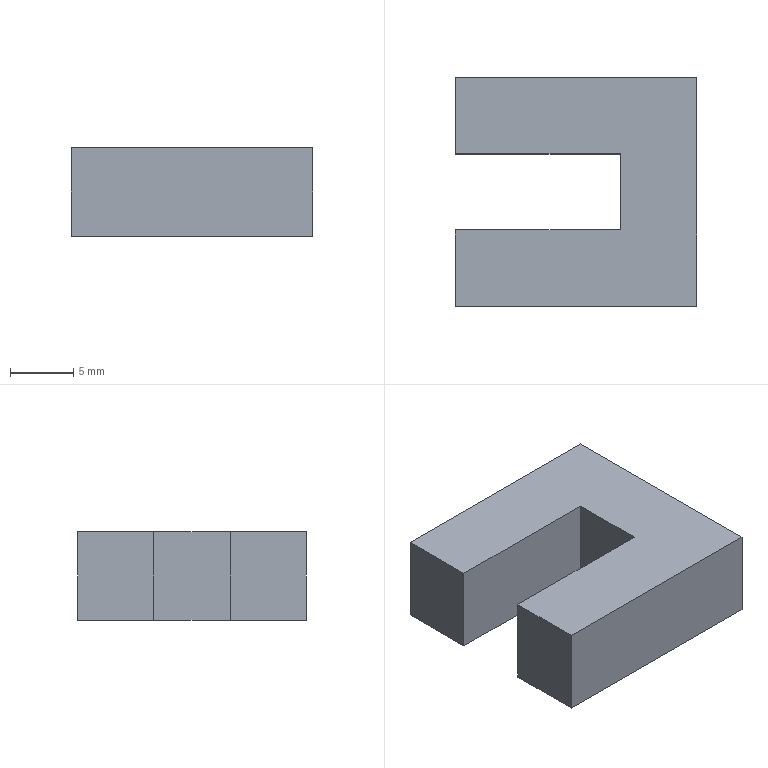Part | SolidWorks | features Extrusion 1 | 1 solid | 10 faces | box 19 x 18 x 7 mm | volume 1848 mm3 | plane 10
STEP:
#1=CARTESIAN_POINT('',(0.,-9.,-3.5));
#2=VERTEX_POINT('',#1);
#3=CARTESIAN_POINT('',(0.,9.,-3.5));
#4=VERTEX_POINT('',#3);
#5=CARTESIAN_POINT('',(0.,0.,-3.5));
#6=DIRECTION('',(0.,1.,0.));
#7=VECTOR('',#6,1000.);
#8=LINE('',#5,#7);
#9=EDGE_CURVE('',#2,#4,#8,.T.);
#10=ORIENTED_EDGE('',*,*,#9,.T.);
#11=CARTESIAN_POINT('',(0.,9.,3.5));
#12=VERTEX_POINT('',#11);
#13=CARTESIAN_POINT('',(0.,9.,3.5));
#14=DIRECTION('',(0.,0.,-1.));
#15=VECTOR('',#14,1000.);
#16=LINE('',#13,#15);
#17=EDGE_CURVE('',#12,#4,#16,.T.);
#18=ORIENTED_EDGE('',*,*,#17,.F.);
#19=CARTESIAN_POINT('',(0.,-9.,3.5));
#20=VERTEX_POINT('',#19);
#21=CARTESIAN_POINT('',(0.,-9.,3.5));
#22=DIRECTION('',(0.,1.,0.));
#23=VECTOR('',#22,1000.);
#24=LINE('',#21,#23);
#25=EDGE_CURVE('',#20,#12,#24,.T.);
#26=ORIENTED_EDGE('',*,*,#25,.F.);
#27=CARTESIAN_POINT('',(0.,-9.,3.5));
#28=DIRECTION('',(0.,0.,-1.));
#29=VECTOR('',#28,1000.);
#30=LINE('',#27,#29);
#31=EDGE_CURVE('',#20,#2,#30,.T.);
#32=ORIENTED_EDGE('',*,*,#31,.T.);
#33=EDGE_LOOP('',(#10,#18,#26,#32));
#34=FACE_OUTER_BOUND('',#33,.T.);
#35=CARTESIAN_POINT('',(0.,0.,3.5));
#36=DIRECTION('',(-1.,0.,0.));
#37=DIRECTION('',(0.,0.,1.));
#38=AXIS2_PLACEMENT_3D('',#35,#36,#37);
#39=PLANE('',#38);
#40=ADVANCED_FACE('',(#34),#39,.F.);
#41=CARTESIAN_POINT('',(-19.,9.,-3.5));
#42=VERTEX_POINT('',#41);
#43=CARTESIAN_POINT('',(0.,9.,-3.5));
#44=DIRECTION('',(-1.,0.,0.));
#45=VECTOR('',#44,1000.);
#46=LINE('',#43,#45);
#47=EDGE_CURVE('',#4,#42,#46,.T.);
#48=ORIENTED_EDGE('',*,*,#47,.T.);
#49=CARTESIAN_POINT('',(-19.,9.,3.5));
#50=VERTEX_POINT('',#49);
#51=CARTESIAN_POINT('',(-19.,9.,3.5));
#52=DIRECTION('',(0.,0.,-1.));
#53=VECTOR('',#52,1000.);
#54=LINE('',#51,#53);
#55=EDGE_CURVE('',#50,#42,#54,.T.);
#56=ORIENTED_EDGE('',*,*,#55,.F.);
#57=CARTESIAN_POINT('',(0.,9.,3.5));
#58=DIRECTION('',(-1.,0.,0.));
#59=VECTOR('',#58,1000.);
#60=LINE('',#57,#59);
#61=EDGE_CURVE('',#12,#50,#60,.T.);
#62=ORIENTED_EDGE('',*,*,#61,.F.);
#63=ORIENTED_EDGE('',*,*,#17,.T.);
#64=EDGE_LOOP('',(#48,#56,#62,#63));
#65=FACE_OUTER_BOUND('',#64,.T.);
#66=CARTESIAN_POINT('',(0.,9.,3.5));
#67=DIRECTION('',(0.,-1.,0.));
#68=DIRECTION('',(1.,0.,0.));
#69=AXIS2_PLACEMENT_3D('',#66,#67,#68);
#70=PLANE('',#69);
#71=ADVANCED_FACE('',(#65),#70,.F.);
#72=CARTESIAN_POINT('',(-19.,3.,-3.5));
#73=VERTEX_POINT('',#72);
#74=CARTESIAN_POINT('',(-19.,9.,-3.5));
#75=DIRECTION('',(0.,-1.,0.));
#76=VECTOR('',#75,1000.);
#77=LINE('',#74,#76);
#78=EDGE_CURVE('',#42,#73,#77,.T.);
#79=ORIENTED_EDGE('',*,*,#78,.T.);
#80=CARTESIAN_POINT('',(-19.,3.,3.5));
#81=VERTEX_POINT('',#80);
#82=CARTESIAN_POINT('',(-19.,3.,3.5));
#83=DIRECTION('',(0.,0.,-1.));
#84=VECTOR('',#83,1000.);
#85=LINE('',#82,#84);
#86=EDGE_CURVE('',#81,#73,#85,.T.);
#87=ORIENTED_EDGE('',*,*,#86,.F.);
#88=CARTESIAN_POINT('',(-19.,9.,3.5));
#89=DIRECTION('',(0.,-1.,0.));
#90=VECTOR('',#89,1000.);
#91=LINE('',#88,#90);
#92=EDGE_CURVE('',#50,#81,#91,.T.);
#93=ORIENTED_EDGE('',*,*,#92,.F.);
#94=ORIENTED_EDGE('',*,*,#55,.T.);
#95=EDGE_LOOP('',(#79,#87,#93,#94));
#96=FACE_OUTER_BOUND('',#95,.T.);
#97=CARTESIAN_POINT('',(-19.,9.,3.5));
#98=DIRECTION('',(1.,0.,0.));
#99=DIRECTION('',(0.,0.,-1.));
#100=AXIS2_PLACEMENT_3D('',#97,#98,#99);
#101=PLANE('',#100);
#102=ADVANCED_FACE('',(#96),#101,.F.);
#103=CARTESIAN_POINT('',(-6.,3.,-3.5));
#104=VERTEX_POINT('',#103);
#105=CARTESIAN_POINT('',(-19.,3.,-3.5));
#106=DIRECTION('',(1.,0.,0.));
#107=VECTOR('',#106,1000.);
#108=LINE('',#105,#107);
#109=EDGE_CURVE('',#73,#104,#108,.T.);
#110=ORIENTED_EDGE('',*,*,#109,.T.);
#111=CARTESIAN_POINT('',(-6.,3.,3.5));
#112=VERTEX_POINT('',#111);
#113=CARTESIAN_POINT('',(-6.,3.,3.5));
#114=DIRECTION('',(0.,0.,-1.));
#115=VECTOR('',#114,1000.);
#116=LINE('',#113,#115);
#117=EDGE_CURVE('',#112,#104,#116,.T.);
#118=ORIENTED_EDGE('',*,*,#117,.F.);
#119=CARTESIAN_POINT('',(-19.,3.,3.5));
#120=DIRECTION('',(1.,0.,0.));
#121=VECTOR('',#120,1000.);
#122=LINE('',#119,#121);
#123=EDGE_CURVE('',#81,#112,#122,.T.);
#124=ORIENTED_EDGE('',*,*,#123,.F.);
#125=ORIENTED_EDGE('',*,*,#86,.T.);
#126=EDGE_LOOP('',(#110,#118,#124,#125));
#127=FACE_OUTER_BOUND('',#126,.T.);
#128=CARTESIAN_POINT('',(-19.,3.,3.5));
#129=DIRECTION('',(0.,1.,0.));
#130=DIRECTION('',(-1.,0.,0.));
#131=AXIS2_PLACEMENT_3D('',#128,#129,#130);
#132=PLANE('',#131);
#133=ADVANCED_FACE('',(#127),#132,.F.);
#134=CARTESIAN_POINT('',(-6.,-3.,-3.5));
#135=VERTEX_POINT('',#134);
#136=CARTESIAN_POINT('',(-6.,3.,-3.5));
#137=DIRECTION('',(0.,-1.,0.));
#138=VECTOR('',#137,1000.);
#139=LINE('',#136,#138);
#140=EDGE_CURVE('',#104,#135,#139,.T.);
#141=ORIENTED_EDGE('',*,*,#140,.T.);
#142=CARTESIAN_POINT('',(-6.,-3.,3.5));
#143=VERTEX_POINT('',#142);
#144=CARTESIAN_POINT('',(-6.,-3.,3.5));
#145=DIRECTION('',(0.,0.,-1.));
#146=VECTOR('',#145,1000.);
#147=LINE('',#144,#146);
#148=EDGE_CURVE('',#143,#135,#147,.T.);
#149=ORIENTED_EDGE('',*,*,#148,.F.);
#150=CARTESIAN_POINT('',(-6.,3.,3.5));
#151=DIRECTION('',(0.,-1.,0.));
#152=VECTOR('',#151,1000.);
#153=LINE('',#150,#152);
#154=EDGE_CURVE('',#112,#143,#153,.T.);
#155=ORIENTED_EDGE('',*,*,#154,.F.);
#156=ORIENTED_EDGE('',*,*,#117,.T.);
#157=EDGE_LOOP('',(#141,#149,#155,#156));
#158=FACE_OUTER_BOUND('',#157,.T.);
#159=CARTESIAN_POINT('',(-6.,3.,3.5));
#160=DIRECTION('',(1.,0.,0.));
#161=DIRECTION('',(0.,1.,0.));
#162=AXIS2_PLACEMENT_3D('',#159,#160,#161);
#163=PLANE('',#162);
#164=ADVANCED_FACE('',(#158),#163,.F.);
#165=CARTESIAN_POINT('',(-19.,-3.,-3.5));
#166=VERTEX_POINT('',#165);
#167=CARTESIAN_POINT('',(-6.,-3.,-3.5));
#168=DIRECTION('',(-1.,0.,0.));
#169=VECTOR('',#168,1000.);
#170=LINE('',#167,#169);
#171=EDGE_CURVE('',#135,#166,#170,.T.);
#172=ORIENTED_EDGE('',*,*,#171,.T.);
#173=CARTESIAN_POINT('',(-19.,-3.,3.5));
#174=VERTEX_POINT('',#173);
#175=CARTESIAN_POINT('',(-19.,-3.,3.5));
#176=DIRECTION('',(0.,0.,-1.));
#177=VECTOR('',#176,1000.);
#178=LINE('',#175,#177);
#179=EDGE_CURVE('',#174,#166,#178,.T.);
#180=ORIENTED_EDGE('',*,*,#179,.F.);
#181=CARTESIAN_POINT('',(-6.,-3.,3.5));
#182=DIRECTION('',(-1.,0.,0.));
#183=VECTOR('',#182,1000.);
#184=LINE('',#181,#183);
#185=EDGE_CURVE('',#143,#174,#184,.T.);
#186=ORIENTED_EDGE('',*,*,#185,.F.);
#187=ORIENTED_EDGE('',*,*,#148,.T.);
#188=EDGE_LOOP('',(#172,#180,#186,#187));
#189=FACE_OUTER_BOUND('',#188,.T.);
#190=CARTESIAN_POINT('',(-6.,-3.,3.5));
#191=DIRECTION('',(0.,-1.,0.));
#192=DIRECTION('',(1.,0.,0.));
#193=AXIS2_PLACEMENT_3D('',#190,#191,#192);
#194=PLANE('',#193);
#195=ADVANCED_FACE('',(#189),#194,.F.);
#196=CARTESIAN_POINT('',(-19.,-9.,-3.5));
#197=VERTEX_POINT('',#196);
#198=CARTESIAN_POINT('',(-19.,-3.,-3.5));
#199=DIRECTION('',(0.,-1.,0.));
#200=VECTOR('',#199,1000.);
#201=LINE('',#198,#200);
#202=EDGE_CURVE('',#166,#197,#201,.T.);
#203=ORIENTED_EDGE('',*,*,#202,.T.);
#204=CARTESIAN_POINT('',(-19.,-9.,3.5));
#205=VERTEX_POINT('',#204);
#206=CARTESIAN_POINT('',(-19.,-9.,3.5));
#207=DIRECTION('',(0.,0.,-1.));
#208=VECTOR('',#207,1000.);
#209=LINE('',#206,#208);
#210=EDGE_CURVE('',#205,#197,#209,.T.);
#211=ORIENTED_EDGE('',*,*,#210,.F.);
#212=CARTESIAN_POINT('',(-19.,-3.,3.5));
#213=DIRECTION('',(0.,-1.,0.));
#214=VECTOR('',#213,1000.);
#215=LINE('',#212,#214);
#216=EDGE_CURVE('',#174,#205,#215,.T.);
#217=ORIENTED_EDGE('',*,*,#216,.F.);
#218=ORIENTED_EDGE('',*,*,#179,.T.);
#219=EDGE_LOOP('',(#203,#211,#217,#218));
#220=FACE_OUTER_BOUND('',#219,.T.);
#221=CARTESIAN_POINT('',(-19.,-3.,3.5));
#222=DIRECTION('',(1.,0.,0.));
#223=DIRECTION('',(0.,0.,-1.));
#224=AXIS2_PLACEMENT_3D('',#221,#222,#223);
#225=PLANE('',#224);
#226=ADVANCED_FACE('',(#220),#225,.F.);
#227=CARTESIAN_POINT('',(-19.,-9.,-3.5));
#228=DIRECTION('',(1.,0.,0.));
#229=VECTOR('',#228,1000.);
#230=LINE('',#227,#229);
#231=EDGE_CURVE('',#197,#2,#230,.T.);
#232=ORIENTED_EDGE('',*,*,#231,.T.);
#233=ORIENTED_EDGE('',*,*,#31,.F.);
#234=CARTESIAN_POINT('',(-19.,-9.,3.5));
#235=DIRECTION('',(1.,0.,0.));
#236=VECTOR('',#235,1000.);
#237=LINE('',#234,#236);
#238=EDGE_CURVE('',#205,#20,#237,.T.);
#239=ORIENTED_EDGE('',*,*,#238,.F.);
#240=ORIENTED_EDGE('',*,*,#210,.T.);
#241=EDGE_LOOP('',(#232,#233,#239,#240));
#242=FACE_OUTER_BOUND('',#241,.T.);
#243=CARTESIAN_POINT('',(-19.,-9.,3.5));
#244=DIRECTION('',(0.,1.,0.));
#245=DIRECTION('',(0.,0.,1.));
#246=AXIS2_PLACEMENT_3D('',#243,#244,#245);
#247=PLANE('',#246);
#248=ADVANCED_FACE('',(#242),#247,.F.);
#249=ORIENTED_EDGE('',*,*,#25,.T.);
#250=ORIENTED_EDGE('',*,*,#61,.T.);
#251=ORIENTED_EDGE('',*,*,#92,.T.);
#252=ORIENTED_EDGE('',*,*,#123,.T.);
#253=ORIENTED_EDGE('',*,*,#154,.T.);
#254=ORIENTED_EDGE('',*,*,#185,.T.);
#255=ORIENTED_EDGE('',*,*,#216,.T.);
#256=ORIENTED_EDGE('',*,*,#238,.T.);
#257=EDGE_LOOP('',(#249,#250,#251,#252,#253,#254,#255,#256));
#258=FACE_OUTER_BOUND('',#257,.T.);
#259=CARTESIAN_POINT('',(0.,0.,3.5));
#260=DIRECTION('',(0.,0.,1.));
#261=DIRECTION('',(1.,0.,0.));
#262=AXIS2_PLACEMENT_3D('',#259,#260,#261);
#263=PLANE('',#262);
#264=ADVANCED_FACE('',(#258),#263,.T.);
#265=ORIENTED_EDGE('',*,*,#9,.F.);
#266=ORIENTED_EDGE('',*,*,#231,.F.);
#267=ORIENTED_EDGE('',*,*,#202,.F.);
#268=ORIENTED_EDGE('',*,*,#171,.F.);
#269=ORIENTED_EDGE('',*,*,#140,.F.);
#270=ORIENTED_EDGE('',*,*,#109,.F.);
#271=ORIENTED_EDGE('',*,*,#78,.F.);
#272=ORIENTED_EDGE('',*,*,#47,.F.);
#273=EDGE_LOOP('',(#265,#266,#267,#268,#269,#270,#271,#272));
#274=FACE_OUTER_BOUND('',#273,.T.);
#275=CARTESIAN_POINT('',(0.,0.,-3.5));
#276=DIRECTION('',(0.,0.,1.));
#277=DIRECTION('',(1.,0.,0.));
#278=AXIS2_PLACEMENT_3D('',#275,#276,#277);
#279=PLANE('',#278);
#280=ADVANCED_FACE('',(#274),#279,.F.);
#281=CLOSED_SHELL('',(#40,#71,#102,#133,#164,#195,#226,#248,#264,#280));
#282=MANIFOLD_SOLID_BREP('',#281);
#283=CARTESIAN_POINT('',(0.,0.,0.));
#284=DIRECTION('',(0.,0.,1.));
#285=DIRECTION('',(1.,0.,0.));
#286=AXIS2_PLACEMENT_3D('',#283,#284,#285);
#287=(LENGTH_UNIT()NAMED_UNIT(*)SI_UNIT(.MILLI.,.METRE.));
#288=UNCERTAINTY_MEASURE_WITH_UNIT(LENGTH_MEASURE(0.00001),#287,'','');
#289=(NAMED_UNIT(*)PLANE_ANGLE_UNIT()SI_UNIT($,.RADIAN.));
#290=(NAMED_UNIT(*)SI_UNIT($,.STERADIAN.)SOLID_ANGLE_UNIT());
#291=(GEOMETRIC_REPRESENTATION_CONTEXT(3)GLOBAL_UNCERTAINTY_ASSIGNED_CONTEXT((#288))GLOBAL_UNIT_ASSIGNED_CONTEXT((#287,#289,#290))REPRESENTATION_CONTEXT('',''));
#292=ADVANCED_BREP_SHAPE_REPRESENTATION('',(#282,#286),#291);